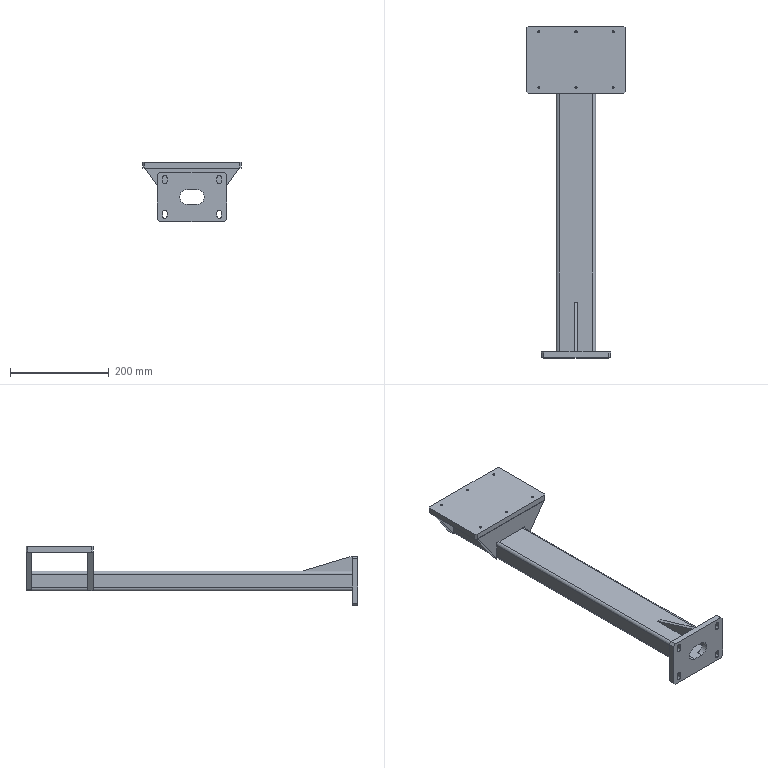Part | STEP file | 0-19-06 Mount seat_Default <Feature> | 4 solids | 108 faces | box 200 x 671.5 x 120 mm | volume 1373687 mm3 | plane 58 | cylinder 44 | cone 6 | commonest cylinder face diameters 4.2 x18 9 x12 2 x4 12 x4 30 x4 10 x2